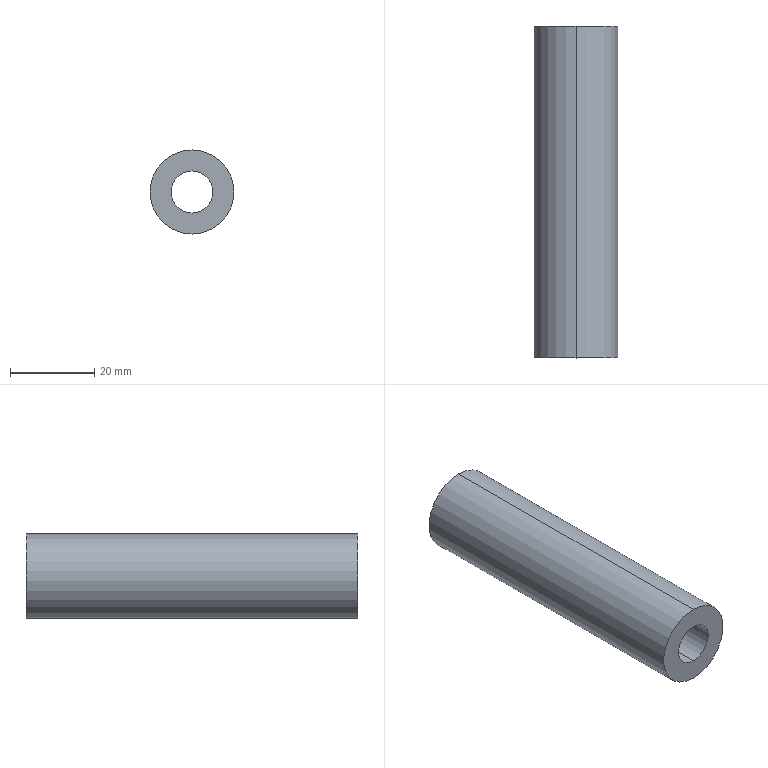Part | SolidWorks | features Extrusion 1 | 1 solid | 6 faces | box 20 x 79 x 20 mm | volume 18614 mm3 | cylinder 4 | plane 2 | commonest cylinder face diameters 10 x2 20 x2
STEP:
#1=CARTESIAN_POINT('',(0.,79.,-5.));
#2=VERTEX_POINT('',#1);
#3=CARTESIAN_POINT('',(0.,79.,5.));
#4=VERTEX_POINT('',#3);
#5=CARTESIAN_POINT('',(0.,79.,0.));
#6=DIRECTION('',(0.,1.,0.));
#7=DIRECTION('',(0.,0.,1.));
#8=AXIS2_PLACEMENT_3D('',#5,#6,#7);
#9=CIRCLE('',#8,5.);
#10=EDGE_CURVE('',#2,#4,#9,.T.);
#11=ORIENTED_EDGE('',*,*,#10,.T.);
#12=CARTESIAN_POINT('',(0.,0.,5.));
#13=VERTEX_POINT('',#12);
#14=CARTESIAN_POINT('',(0.,79.,5.));
#15=DIRECTION('',(0.,-1.,0.));
#16=VECTOR('',#15,1000.);
#17=LINE('',#14,#16);
#18=EDGE_CURVE('',#4,#13,#17,.T.);
#19=ORIENTED_EDGE('',*,*,#18,.T.);
#20=CARTESIAN_POINT('',(0.,0.,-5.));
#21=VERTEX_POINT('',#20);
#22=CARTESIAN_POINT('',(0.,0.,0.));
#23=DIRECTION('',(0.,1.,0.));
#24=DIRECTION('',(0.,0.,1.));
#25=AXIS2_PLACEMENT_3D('',#22,#23,#24);
#26=CIRCLE('',#25,5.);
#27=EDGE_CURVE('',#21,#13,#26,.T.);
#28=ORIENTED_EDGE('',*,*,#27,.F.);
#29=CARTESIAN_POINT('',(0.,79.,-5.));
#30=DIRECTION('',(0.,-1.,0.));
#31=VECTOR('',#30,1000.);
#32=LINE('',#29,#31);
#33=EDGE_CURVE('',#2,#21,#32,.T.);
#34=ORIENTED_EDGE('',*,*,#33,.F.);
#35=EDGE_LOOP('',(#11,#19,#28,#34));
#36=FACE_OUTER_BOUND('',#35,.T.);
#37=CARTESIAN_POINT('',(0.,79.,0.));
#38=DIRECTION('',(0.,-1.,0.));
#39=DIRECTION('',(0.,0.,-1.));
#40=AXIS2_PLACEMENT_3D('',#37,#38,#39);
#41=CYLINDRICAL_SURFACE('',#40,5.);
#42=ADVANCED_FACE('',(#36),#41,.F.);
#43=CARTESIAN_POINT('',(0.,79.,10.));
#44=VERTEX_POINT('',#43);
#45=CARTESIAN_POINT('',(0.,79.,-10.));
#46=VERTEX_POINT('',#45);
#47=CARTESIAN_POINT('',(0.,79.,0.));
#48=DIRECTION('',(0.,1.,0.));
#49=DIRECTION('',(0.,0.,1.));
#50=AXIS2_PLACEMENT_3D('',#47,#48,#49);
#51=CIRCLE('',#50,10.);
#52=EDGE_CURVE('',#44,#46,#51,.T.);
#53=ORIENTED_EDGE('',*,*,#52,.F.);
#54=CARTESIAN_POINT('',(0.,0.,10.));
#55=VERTEX_POINT('',#54);
#56=CARTESIAN_POINT('',(0.,79.,10.));
#57=DIRECTION('',(0.,-1.,0.));
#58=VECTOR('',#57,1000.);
#59=LINE('',#56,#58);
#60=EDGE_CURVE('',#44,#55,#59,.T.);
#61=ORIENTED_EDGE('',*,*,#60,.T.);
#62=CARTESIAN_POINT('',(0.,0.,-10.));
#63=VERTEX_POINT('',#62);
#64=CARTESIAN_POINT('',(0.,0.,0.));
#65=DIRECTION('',(0.,1.,0.));
#66=DIRECTION('',(0.,0.,1.));
#67=AXIS2_PLACEMENT_3D('',#64,#65,#66);
#68=CIRCLE('',#67,10.);
#69=EDGE_CURVE('',#55,#63,#68,.T.);
#70=ORIENTED_EDGE('',*,*,#69,.T.);
#71=CARTESIAN_POINT('',(0.,79.,-10.));
#72=DIRECTION('',(0.,-1.,0.));
#73=VECTOR('',#72,1000.);
#74=LINE('',#71,#73);
#75=EDGE_CURVE('',#46,#63,#74,.T.);
#76=ORIENTED_EDGE('',*,*,#75,.F.);
#77=EDGE_LOOP('',(#53,#61,#70,#76));
#78=FACE_OUTER_BOUND('',#77,.T.);
#79=CARTESIAN_POINT('',(0.,79.,0.));
#80=DIRECTION('',(0.,-1.,0.));
#81=DIRECTION('',(0.,0.,-1.));
#82=AXIS2_PLACEMENT_3D('',#79,#80,#81);
#83=CYLINDRICAL_SURFACE('',#82,10.);
#84=ADVANCED_FACE('',(#78),#83,.T.);
#85=CARTESIAN_POINT('',(0.,79.,0.));
#86=DIRECTION('',(0.,1.,0.));
#87=DIRECTION('',(0.,0.,1.));
#88=AXIS2_PLACEMENT_3D('',#85,#86,#87);
#89=CIRCLE('',#88,10.);
#90=EDGE_CURVE('',#46,#44,#89,.T.);
#91=ORIENTED_EDGE('',*,*,#90,.T.);
#92=ORIENTED_EDGE('',*,*,#52,.T.);
#93=EDGE_LOOP('',(#91,#92));
#94=FACE_OUTER_BOUND('',#93,.T.);
#95=ORIENTED_EDGE('',*,*,#10,.F.);
#96=CARTESIAN_POINT('',(0.,79.,0.));
#97=DIRECTION('',(0.,1.,0.));
#98=DIRECTION('',(0.,0.,1.));
#99=AXIS2_PLACEMENT_3D('',#96,#97,#98);
#100=CIRCLE('',#99,5.);
#101=EDGE_CURVE('',#4,#2,#100,.T.);
#102=ORIENTED_EDGE('',*,*,#101,.F.);
#103=EDGE_LOOP('',(#95,#102));
#104=FACE_BOUND('',#103,.T.);
#105=CARTESIAN_POINT('',(0.,79.,0.));
#106=DIRECTION('',(0.,1.,0.));
#107=DIRECTION('',(0.,0.,1.));
#108=AXIS2_PLACEMENT_3D('',#105,#106,#107);
#109=PLANE('',#108);
#110=ADVANCED_FACE('',(#94,#104),#109,.T.);
#111=CARTESIAN_POINT('',(0.,0.,0.));
#112=DIRECTION('',(0.,1.,0.));
#113=DIRECTION('',(0.,0.,1.));
#114=AXIS2_PLACEMENT_3D('',#111,#112,#113);
#115=CIRCLE('',#114,10.);
#116=EDGE_CURVE('',#63,#55,#115,.T.);
#117=ORIENTED_EDGE('',*,*,#116,.F.);
#118=ORIENTED_EDGE('',*,*,#69,.F.);
#119=EDGE_LOOP('',(#117,#118));
#120=FACE_OUTER_BOUND('',#119,.T.);
#121=ORIENTED_EDGE('',*,*,#27,.T.);
#122=CARTESIAN_POINT('',(0.,0.,0.));
#123=DIRECTION('',(0.,1.,0.));
#124=DIRECTION('',(0.,0.,1.));
#125=AXIS2_PLACEMENT_3D('',#122,#123,#124);
#126=CIRCLE('',#125,5.);
#127=EDGE_CURVE('',#13,#21,#126,.T.);
#128=ORIENTED_EDGE('',*,*,#127,.T.);
#129=EDGE_LOOP('',(#121,#128));
#130=FACE_BOUND('',#129,.T.);
#131=CARTESIAN_POINT('',(0.,0.,0.));
#132=DIRECTION('',(0.,1.,0.));
#133=DIRECTION('',(0.,0.,1.));
#134=AXIS2_PLACEMENT_3D('',#131,#132,#133);
#135=PLANE('',#134);
#136=ADVANCED_FACE('',(#120,#130),#135,.F.);
#137=ORIENTED_EDGE('',*,*,#60,.F.);
#138=ORIENTED_EDGE('',*,*,#90,.F.);
#139=ORIENTED_EDGE('',*,*,#75,.T.);
#140=ORIENTED_EDGE('',*,*,#116,.T.);
#141=EDGE_LOOP('',(#137,#138,#139,#140));
#142=FACE_OUTER_BOUND('',#141,.T.);
#143=CARTESIAN_POINT('',(0.,79.,0.));
#144=DIRECTION('',(0.,-1.,0.));
#145=DIRECTION('',(0.,0.,-1.));
#146=AXIS2_PLACEMENT_3D('',#143,#144,#145);
#147=CYLINDRICAL_SURFACE('',#146,10.);
#148=ADVANCED_FACE('',(#142),#147,.T.);
#149=ORIENTED_EDGE('',*,*,#18,.F.);
#150=ORIENTED_EDGE('',*,*,#101,.T.);
#151=ORIENTED_EDGE('',*,*,#33,.T.);
#152=ORIENTED_EDGE('',*,*,#127,.F.);
#153=EDGE_LOOP('',(#149,#150,#151,#152));
#154=FACE_OUTER_BOUND('',#153,.T.);
#155=CARTESIAN_POINT('',(0.,79.,0.));
#156=DIRECTION('',(0.,-1.,0.));
#157=DIRECTION('',(0.,0.,-1.));
#158=AXIS2_PLACEMENT_3D('',#155,#156,#157);
#159=CYLINDRICAL_SURFACE('',#158,5.);
#160=ADVANCED_FACE('',(#154),#159,.F.);
#161=CLOSED_SHELL('',(#42,#84,#110,#136,#148,#160));
#162=MANIFOLD_SOLID_BREP('',#161);
#163=CARTESIAN_POINT('',(0.,0.,0.));
#164=DIRECTION('',(0.,0.,1.));
#165=DIRECTION('',(1.,0.,0.));
#166=AXIS2_PLACEMENT_3D('',#163,#164,#165);
#167=(LENGTH_UNIT()NAMED_UNIT(*)SI_UNIT(.MILLI.,.METRE.));
#168=UNCERTAINTY_MEASURE_WITH_UNIT(LENGTH_MEASURE(0.00001),#167,'','');
#169=(NAMED_UNIT(*)PLANE_ANGLE_UNIT()SI_UNIT($,.RADIAN.));
#170=(NAMED_UNIT(*)SI_UNIT($,.STERADIAN.)SOLID_ANGLE_UNIT());
#171=(GEOMETRIC_REPRESENTATION_CONTEXT(3)GLOBAL_UNCERTAINTY_ASSIGNED_CONTEXT((#168))GLOBAL_UNIT_ASSIGNED_CONTEXT((#167,#169,#170))REPRESENTATION_CONTEXT('',''));
#172=ADVANCED_BREP_SHAPE_REPRESENTATION('',(#162,#166),#171);